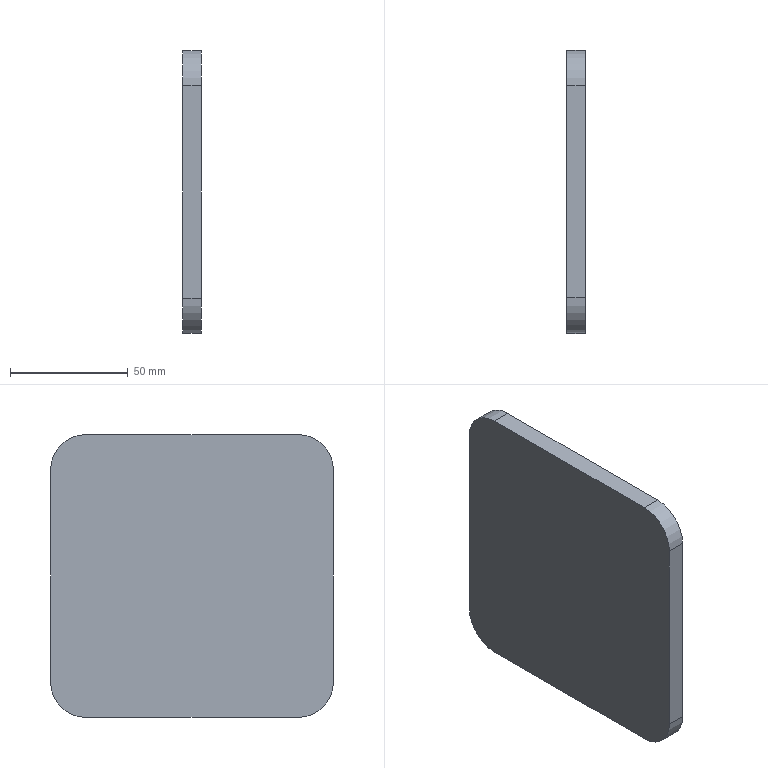Part | SolidWorks | features BaseBody 1 | 1 solid | 10 faces | box 8 x 120 x 120 mm | volume 113655 mm3 | plane 6 | cylinder 4 | commonest cylinder face diameters 30 x4
STEP:
#1=CARTESIAN_POINT('',(8.,-45.,60.));
#2=VERTEX_POINT('',#1);
#3=CARTESIAN_POINT('',(8.,-60.,45.));
#4=VERTEX_POINT('',#3);
#5=CARTESIAN_POINT('',(8.,-45.,45.));
#6=DIRECTION('',(1.,0.,0.));
#7=DIRECTION('',(0.,0.,1.));
#8=AXIS2_PLACEMENT_3D('',#5,#6,#7);
#9=CIRCLE('',#8,15.);
#10=EDGE_CURVE('',#2,#4,#9,.T.);
#11=ORIENTED_EDGE('',*,*,#10,.F.);
#12=CARTESIAN_POINT('',(0.,-45.,60.));
#13=VERTEX_POINT('',#12);
#14=CARTESIAN_POINT('',(8.,-45.,60.));
#15=DIRECTION('',(1.,0.,0.));
#16=VECTOR('',#15,1000.);
#17=LINE('',#14,#16);
#18=EDGE_CURVE('',#13,#2,#17,.T.);
#19=ORIENTED_EDGE('',*,*,#18,.F.);
#20=CARTESIAN_POINT('',(0.,-60.,45.));
#21=VERTEX_POINT('',#20);
#22=CARTESIAN_POINT('',(0.,-45.,45.));
#23=DIRECTION('',(-1.,0.,0.));
#24=DIRECTION('',(0.,0.,1.));
#25=AXIS2_PLACEMENT_3D('',#22,#23,#24);
#26=CIRCLE('',#25,15.);
#27=EDGE_CURVE('',#21,#13,#26,.T.);
#28=ORIENTED_EDGE('',*,*,#27,.F.);
#29=CARTESIAN_POINT('',(8.,-60.,45.));
#30=DIRECTION('',(-1.,0.,0.));
#31=VECTOR('',#30,1000.);
#32=LINE('',#29,#31);
#33=EDGE_CURVE('',#4,#21,#32,.T.);
#34=ORIENTED_EDGE('',*,*,#33,.F.);
#35=EDGE_LOOP('',(#11,#19,#28,#34));
#36=FACE_OUTER_BOUND('',#35,.T.);
#37=CARTESIAN_POINT('',(8.,-45.,45.));
#38=DIRECTION('',(-1.,0.,0.));
#39=DIRECTION('',(0.,0.,1.));
#40=AXIS2_PLACEMENT_3D('',#37,#38,#39);
#41=CYLINDRICAL_SURFACE('',#40,15.);
#42=ADVANCED_FACE('',(#36),#41,.T.);
#43=CARTESIAN_POINT('',(8.,-60.,-45.));
#44=VERTEX_POINT('',#43);
#45=CARTESIAN_POINT('',(8.,-45.,-60.));
#46=VERTEX_POINT('',#45);
#47=CARTESIAN_POINT('',(8.,-45.,-45.));
#48=DIRECTION('',(1.,0.,0.));
#49=DIRECTION('',(0.,0.,1.));
#50=AXIS2_PLACEMENT_3D('',#47,#48,#49);
#51=CIRCLE('',#50,15.);
#52=EDGE_CURVE('',#44,#46,#51,.T.);
#53=ORIENTED_EDGE('',*,*,#52,.F.);
#54=CARTESIAN_POINT('',(0.,-60.,-45.));
#55=VERTEX_POINT('',#54);
#56=CARTESIAN_POINT('',(8.,-60.,-45.));
#57=DIRECTION('',(1.,0.,0.));
#58=VECTOR('',#57,1000.);
#59=LINE('',#56,#58);
#60=EDGE_CURVE('',#55,#44,#59,.T.);
#61=ORIENTED_EDGE('',*,*,#60,.F.);
#62=CARTESIAN_POINT('',(0.,-45.,-60.));
#63=VERTEX_POINT('',#62);
#64=CARTESIAN_POINT('',(0.,-45.,-45.));
#65=DIRECTION('',(-1.,0.,0.));
#66=DIRECTION('',(0.,0.,1.));
#67=AXIS2_PLACEMENT_3D('',#64,#65,#66);
#68=CIRCLE('',#67,15.);
#69=EDGE_CURVE('',#63,#55,#68,.T.);
#70=ORIENTED_EDGE('',*,*,#69,.F.);
#71=CARTESIAN_POINT('',(8.,-45.,-60.));
#72=DIRECTION('',(-1.,0.,0.));
#73=VECTOR('',#72,1000.);
#74=LINE('',#71,#73);
#75=EDGE_CURVE('',#46,#63,#74,.T.);
#76=ORIENTED_EDGE('',*,*,#75,.F.);
#77=EDGE_LOOP('',(#53,#61,#70,#76));
#78=FACE_OUTER_BOUND('',#77,.T.);
#79=CARTESIAN_POINT('',(8.,-45.,-45.));
#80=DIRECTION('',(-1.,0.,0.));
#81=DIRECTION('',(0.,0.,1.));
#82=AXIS2_PLACEMENT_3D('',#79,#80,#81);
#83=CYLINDRICAL_SURFACE('',#82,15.);
#84=ADVANCED_FACE('',(#78),#83,.T.);
#85=CARTESIAN_POINT('',(8.,45.,-60.));
#86=VERTEX_POINT('',#85);
#87=CARTESIAN_POINT('',(8.,60.,-45.));
#88=VERTEX_POINT('',#87);
#89=CARTESIAN_POINT('',(8.,45.,-45.));
#90=DIRECTION('',(1.,0.,0.));
#91=DIRECTION('',(0.,0.,1.));
#92=AXIS2_PLACEMENT_3D('',#89,#90,#91);
#93=CIRCLE('',#92,15.);
#94=EDGE_CURVE('',#86,#88,#93,.T.);
#95=ORIENTED_EDGE('',*,*,#94,.F.);
#96=CARTESIAN_POINT('',(0.,45.,-60.));
#97=VERTEX_POINT('',#96);
#98=CARTESIAN_POINT('',(8.,45.,-60.));
#99=DIRECTION('',(1.,0.,0.));
#100=VECTOR('',#99,1000.);
#101=LINE('',#98,#100);
#102=EDGE_CURVE('',#97,#86,#101,.T.);
#103=ORIENTED_EDGE('',*,*,#102,.F.);
#104=CARTESIAN_POINT('',(0.,60.,-45.));
#105=VERTEX_POINT('',#104);
#106=CARTESIAN_POINT('',(0.,45.,-45.));
#107=DIRECTION('',(-1.,0.,0.));
#108=DIRECTION('',(0.,0.,1.));
#109=AXIS2_PLACEMENT_3D('',#106,#107,#108);
#110=CIRCLE('',#109,15.);
#111=EDGE_CURVE('',#105,#97,#110,.T.);
#112=ORIENTED_EDGE('',*,*,#111,.F.);
#113=CARTESIAN_POINT('',(8.,60.,-45.));
#114=DIRECTION('',(-1.,0.,0.));
#115=VECTOR('',#114,1000.);
#116=LINE('',#113,#115);
#117=EDGE_CURVE('',#88,#105,#116,.T.);
#118=ORIENTED_EDGE('',*,*,#117,.F.);
#119=EDGE_LOOP('',(#95,#103,#112,#118));
#120=FACE_OUTER_BOUND('',#119,.T.);
#121=CARTESIAN_POINT('',(8.,45.,-45.));
#122=DIRECTION('',(-1.,0.,0.));
#123=DIRECTION('',(0.,0.,1.));
#124=AXIS2_PLACEMENT_3D('',#121,#122,#123);
#125=CYLINDRICAL_SURFACE('',#124,15.);
#126=ADVANCED_FACE('',(#120),#125,.T.);
#127=CARTESIAN_POINT('',(8.,60.,45.));
#128=VERTEX_POINT('',#127);
#129=CARTESIAN_POINT('',(8.,45.,60.));
#130=VERTEX_POINT('',#129);
#131=CARTESIAN_POINT('',(8.,45.,45.));
#132=DIRECTION('',(1.,0.,0.));
#133=DIRECTION('',(0.,0.,1.));
#134=AXIS2_PLACEMENT_3D('',#131,#132,#133);
#135=CIRCLE('',#134,15.);
#136=EDGE_CURVE('',#128,#130,#135,.T.);
#137=ORIENTED_EDGE('',*,*,#136,.F.);
#138=CARTESIAN_POINT('',(0.,60.,45.));
#139=VERTEX_POINT('',#138);
#140=CARTESIAN_POINT('',(8.,60.,45.));
#141=DIRECTION('',(1.,0.,0.));
#142=VECTOR('',#141,1000.);
#143=LINE('',#140,#142);
#144=EDGE_CURVE('',#139,#128,#143,.T.);
#145=ORIENTED_EDGE('',*,*,#144,.F.);
#146=CARTESIAN_POINT('',(0.,45.,60.));
#147=VERTEX_POINT('',#146);
#148=CARTESIAN_POINT('',(0.,45.,45.));
#149=DIRECTION('',(-1.,0.,0.));
#150=DIRECTION('',(0.,0.,1.));
#151=AXIS2_PLACEMENT_3D('',#148,#149,#150);
#152=CIRCLE('',#151,15.);
#153=EDGE_CURVE('',#147,#139,#152,.T.);
#154=ORIENTED_EDGE('',*,*,#153,.F.);
#155=CARTESIAN_POINT('',(8.,45.,60.));
#156=DIRECTION('',(-1.,0.,0.));
#157=VECTOR('',#156,1000.);
#158=LINE('',#155,#157);
#159=EDGE_CURVE('',#130,#147,#158,.T.);
#160=ORIENTED_EDGE('',*,*,#159,.F.);
#161=EDGE_LOOP('',(#137,#145,#154,#160));
#162=FACE_OUTER_BOUND('',#161,.T.);
#163=CARTESIAN_POINT('',(8.,45.,45.));
#164=DIRECTION('',(-1.,0.,0.));
#165=DIRECTION('',(0.,0.,1.));
#166=AXIS2_PLACEMENT_3D('',#163,#164,#165);
#167=CYLINDRICAL_SURFACE('',#166,15.);
#168=ADVANCED_FACE('',(#162),#167,.T.);
#169=CARTESIAN_POINT('',(0.,-60.,60.));
#170=DIRECTION('',(0.,-1.,0.));
#171=VECTOR('',#170,1000.);
#172=LINE('',#169,#171);
#173=EDGE_CURVE('',#147,#13,#172,.T.);
#174=ORIENTED_EDGE('',*,*,#173,.F.);
#175=ORIENTED_EDGE('',*,*,#153,.T.);
#176=CARTESIAN_POINT('',(0.,60.,60.));
#177=DIRECTION('',(0.,0.,1.));
#178=VECTOR('',#177,1000.);
#179=LINE('',#176,#178);
#180=EDGE_CURVE('',#105,#139,#179,.T.);
#181=ORIENTED_EDGE('',*,*,#180,.F.);
#182=ORIENTED_EDGE('',*,*,#111,.T.);
#183=CARTESIAN_POINT('',(0.,-60.,-60.));
#184=DIRECTION('',(0.,1.,0.));
#185=VECTOR('',#184,1000.);
#186=LINE('',#183,#185);
#187=EDGE_CURVE('',#63,#97,#186,.T.);
#188=ORIENTED_EDGE('',*,*,#187,.F.);
#189=ORIENTED_EDGE('',*,*,#69,.T.);
#190=CARTESIAN_POINT('',(0.,-60.,60.));
#191=DIRECTION('',(0.,0.,-1.));
#192=VECTOR('',#191,1000.);
#193=LINE('',#190,#192);
#194=EDGE_CURVE('',#21,#55,#193,.T.);
#195=ORIENTED_EDGE('',*,*,#194,.F.);
#196=ORIENTED_EDGE('',*,*,#27,.T.);
#197=EDGE_LOOP('',(#174,#175,#181,#182,#188,#189,#195,#196));
#198=FACE_OUTER_BOUND('',#197,.T.);
#199=CARTESIAN_POINT('',(0.,0.,0.));
#200=DIRECTION('',(-1.,0.,0.));
#201=DIRECTION('',(0.,0.,1.));
#202=AXIS2_PLACEMENT_3D('',#199,#200,#201);
#203=PLANE('',#202);
#204=ADVANCED_FACE('',(#198),#203,.T.);
#205=CARTESIAN_POINT('',(8.,60.,60.));
#206=DIRECTION('',(0.,0.,1.));
#207=VECTOR('',#206,1000.);
#208=LINE('',#205,#207);
#209=EDGE_CURVE('',#88,#128,#208,.T.);
#210=ORIENTED_EDGE('',*,*,#209,.T.);
#211=ORIENTED_EDGE('',*,*,#136,.T.);
#212=CARTESIAN_POINT('',(8.,-60.,60.));
#213=DIRECTION('',(0.,-1.,0.));
#214=VECTOR('',#213,1000.);
#215=LINE('',#212,#214);
#216=EDGE_CURVE('',#130,#2,#215,.T.);
#217=ORIENTED_EDGE('',*,*,#216,.T.);
#218=ORIENTED_EDGE('',*,*,#10,.T.);
#219=CARTESIAN_POINT('',(8.,-60.,60.));
#220=DIRECTION('',(0.,0.,-1.));
#221=VECTOR('',#220,1000.);
#222=LINE('',#219,#221);
#223=EDGE_CURVE('',#4,#44,#222,.T.);
#224=ORIENTED_EDGE('',*,*,#223,.T.);
#225=ORIENTED_EDGE('',*,*,#52,.T.);
#226=CARTESIAN_POINT('',(8.,-60.,-60.));
#227=DIRECTION('',(0.,1.,0.));
#228=VECTOR('',#227,1000.);
#229=LINE('',#226,#228);
#230=EDGE_CURVE('',#46,#86,#229,.T.);
#231=ORIENTED_EDGE('',*,*,#230,.T.);
#232=ORIENTED_EDGE('',*,*,#94,.T.);
#233=EDGE_LOOP('',(#210,#211,#217,#218,#224,#225,#231,#232));
#234=FACE_OUTER_BOUND('',#233,.T.);
#235=CARTESIAN_POINT('',(8.,0.,0.));
#236=DIRECTION('',(-1.,0.,0.));
#237=DIRECTION('',(0.,0.,1.));
#238=AXIS2_PLACEMENT_3D('',#235,#236,#237);
#239=PLANE('',#238);
#240=ADVANCED_FACE('',(#234),#239,.F.);
#241=ORIENTED_EDGE('',*,*,#194,.T.);
#242=ORIENTED_EDGE('',*,*,#60,.T.);
#243=ORIENTED_EDGE('',*,*,#223,.F.);
#244=ORIENTED_EDGE('',*,*,#33,.T.);
#245=EDGE_LOOP('',(#241,#242,#243,#244));
#246=FACE_OUTER_BOUND('',#245,.T.);
#247=CARTESIAN_POINT('',(8.,-60.,60.));
#248=DIRECTION('',(0.,1.,0.));
#249=DIRECTION('',(1.,0.,0.));
#250=AXIS2_PLACEMENT_3D('',#247,#248,#249);
#251=PLANE('',#250);
#252=ADVANCED_FACE('',(#246),#251,.F.);
#253=ORIENTED_EDGE('',*,*,#216,.F.);
#254=ORIENTED_EDGE('',*,*,#159,.T.);
#255=ORIENTED_EDGE('',*,*,#173,.T.);
#256=ORIENTED_EDGE('',*,*,#18,.T.);
#257=EDGE_LOOP('',(#253,#254,#255,#256));
#258=FACE_OUTER_BOUND('',#257,.T.);
#259=CARTESIAN_POINT('',(8.,-60.,60.));
#260=DIRECTION('',(0.,0.,-1.));
#261=DIRECTION('',(0.,-1.,0.));
#262=AXIS2_PLACEMENT_3D('',#259,#260,#261);
#263=PLANE('',#262);
#264=ADVANCED_FACE('',(#258),#263,.F.);
#265=ORIENTED_EDGE('',*,*,#180,.T.);
#266=ORIENTED_EDGE('',*,*,#144,.T.);
#267=ORIENTED_EDGE('',*,*,#209,.F.);
#268=ORIENTED_EDGE('',*,*,#117,.T.);
#269=EDGE_LOOP('',(#265,#266,#267,#268));
#270=FACE_OUTER_BOUND('',#269,.T.);
#271=CARTESIAN_POINT('',(8.,60.,60.));
#272=DIRECTION('',(0.,-1.,0.));
#273=DIRECTION('',(0.,0.,-1.));
#274=AXIS2_PLACEMENT_3D('',#271,#272,#273);
#275=PLANE('',#274);
#276=ADVANCED_FACE('',(#270),#275,.F.);
#277=ORIENTED_EDGE('',*,*,#187,.T.);
#278=ORIENTED_EDGE('',*,*,#102,.T.);
#279=ORIENTED_EDGE('',*,*,#230,.F.);
#280=ORIENTED_EDGE('',*,*,#75,.T.);
#281=EDGE_LOOP('',(#277,#278,#279,#280));
#282=FACE_OUTER_BOUND('',#281,.T.);
#283=CARTESIAN_POINT('',(8.,-60.,-60.));
#284=DIRECTION('',(0.,0.,1.));
#285=DIRECTION('',(1.,0.,0.));
#286=AXIS2_PLACEMENT_3D('',#283,#284,#285);
#287=PLANE('',#286);
#288=ADVANCED_FACE('',(#282),#287,.F.);
#289=CLOSED_SHELL('',(#42,#84,#126,#168,#204,#240,#252,#264,#276,#288));
#290=MANIFOLD_SOLID_BREP('',#289);
#291=CARTESIAN_POINT('',(0.,0.,0.));
#292=DIRECTION('',(0.,0.,1.));
#293=DIRECTION('',(1.,0.,0.));
#294=AXIS2_PLACEMENT_3D('',#291,#292,#293);
#295=(LENGTH_UNIT()NAMED_UNIT(*)SI_UNIT(.MILLI.,.METRE.));
#296=UNCERTAINTY_MEASURE_WITH_UNIT(LENGTH_MEASURE(0.00001),#295,'','');
#297=(NAMED_UNIT(*)PLANE_ANGLE_UNIT()SI_UNIT($,.RADIAN.));
#298=(NAMED_UNIT(*)SI_UNIT($,.STERADIAN.)SOLID_ANGLE_UNIT());
#299=(GEOMETRIC_REPRESENTATION_CONTEXT(3)GLOBAL_UNCERTAINTY_ASSIGNED_CONTEXT((#296))GLOBAL_UNIT_ASSIGNED_CONTEXT((#295,#297,#298))REPRESENTATION_CONTEXT('',''));
#300=ADVANCED_BREP_SHAPE_REPRESENTATION('',(#290,#294),#299);